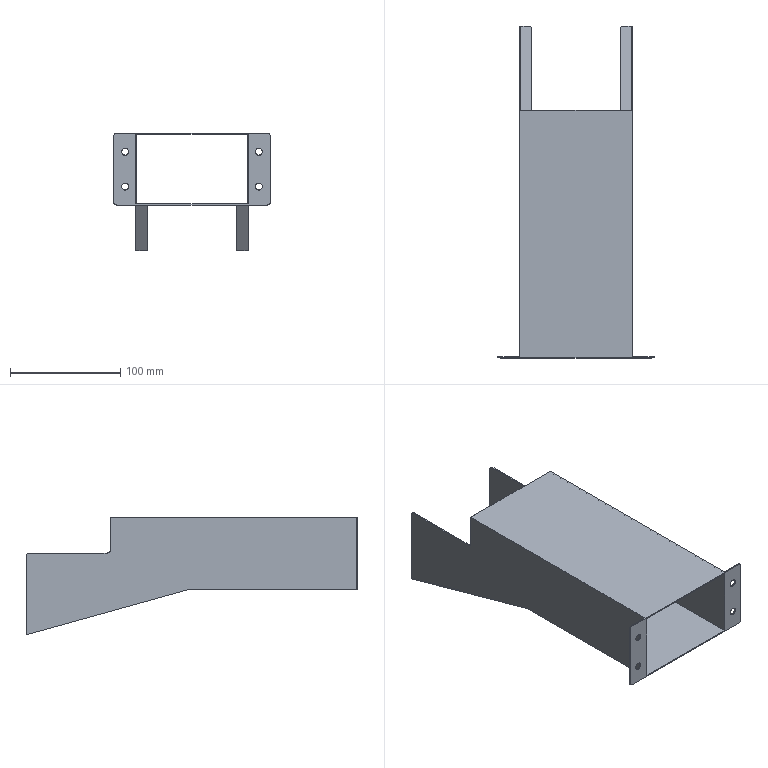Part | NX | 1 solid | 51 faces | box 142 x 300.6 x 106.444 mm | volume 82472 mm3 | plane 25 | cylinder 18 | cone 8 | commonest cylinder face diameters 6 x18